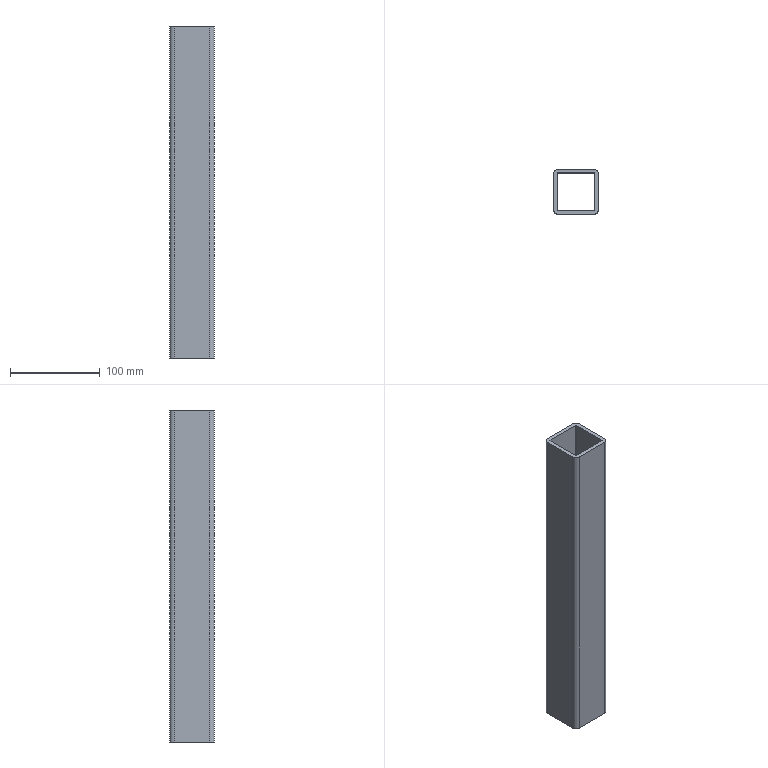Part | STEP file | Square steel 50×50×370 | 1 solid | 18 faces | box 50 x 50 x 370 mm | volume 264697 mm3 | plane 10 | cylinder 8 | commonest cylinder face diameters 2 x4 10 x4
STEP:
#1=CARTESIAN_POINT('',(0.,0.,0.));
#2=DIRECTION('',(0.,0.,1.));
#3=DIRECTION('',(1.,0.,0.));
#4=AXIS2_PLACEMENT_3D('',#1,#2,#3);
#5=CARTESIAN_POINT('',(-25.,-20.,185.));
#6=VERTEX_POINT('',#5);
#7=CARTESIAN_POINT('',(-20.,-25.,185.));
#8=VERTEX_POINT('',#7);
#9=CARTESIAN_POINT('',(-20.,-20.,185.));
#10=DIRECTION('',(0.,0.,1.));
#11=DIRECTION('',(1.,0.,0.));
#12=AXIS2_PLACEMENT_3D('',#9,#10,#11);
#13=CIRCLE('',#12,5.);
#14=CARTESIAN_POINT('',(-20.,-20.,185.));
#15=DIRECTION('',(0.,0.,1.));
#16=DIRECTION('',(1.,0.,0.));
#17=AXIS2_PLACEMENT_3D('',#14,#15,#16);
#18=PLANE('',#17);
#19=CARTESIAN_POINT('',(0.,0.));
#20=DIRECTION('',(1.,0.));
#21=AXIS2_PLACEMENT_2D('',#19,#20);
#22=CIRCLE('',#21,5.);
#23=(GEOMETRIC_REPRESENTATION_CONTEXT(2)PARAMETRIC_REPRESENTATION_CONTEXT()REPRESENTATION_CONTEXT('',''));
#24=DEFINITIONAL_REPRESENTATION('',(#22),#23);
#25=PCURVE('',#18,#24);
#26=CARTESIAN_POINT('',(-20.,-20.,185.));
#27=DIRECTION('',(0.,0.,-1.));
#28=DIRECTION('',(-1.,0.,0.));
#29=AXIS2_PLACEMENT_3D('',#26,#27,#28);
#30=CYLINDRICAL_SURFACE('',#29,5.);
#31=CARTESIAN_POINT('',(9.425,0.));
#32=DIRECTION('',(-1.,0.));
#33=VECTOR('',#32,1.);
#34=LINE('',#31,#33);
#35=(GEOMETRIC_REPRESENTATION_CONTEXT(2)PARAMETRIC_REPRESENTATION_CONTEXT()REPRESENTATION_CONTEXT('',''));
#36=DEFINITIONAL_REPRESENTATION('',(#34),#35);
#37=PCURVE('',#30,#36);
#38=SURFACE_CURVE('',#13,(#25,#37),.PCURVE_S1.);
#39=EDGE_CURVE('',#6,#8,#38,.T.);
#40=ORIENTED_EDGE('',*,*,#39,.T.);
#41=CARTESIAN_POINT('',(20.,-25.,185.));
#42=VERTEX_POINT('',#41);
#43=CARTESIAN_POINT('',(-20.,-25.,185.));
#44=DIRECTION('',(1.,0.,0.));
#45=VECTOR('',#44,1.);
#46=LINE('',#43,#45);
#47=CARTESIAN_POINT('',(0.,-5.));
#48=DIRECTION('',(1.,0.));
#49=VECTOR('',#48,1.);
#50=LINE('',#47,#49);
#51=(GEOMETRIC_REPRESENTATION_CONTEXT(2)PARAMETRIC_REPRESENTATION_CONTEXT()REPRESENTATION_CONTEXT('',''));
#52=DEFINITIONAL_REPRESENTATION('',(#50),#51);
#53=PCURVE('',#18,#52);
#54=CARTESIAN_POINT('',(-20.,-25.,185.));
#55=DIRECTION('',(0.,1.,0.));
#56=DIRECTION('',(0.,0.,1.));
#57=AXIS2_PLACEMENT_3D('',#54,#55,#56);
#58=PLANE('',#57);
#59=CARTESIAN_POINT('',(0.,0.));
#60=DIRECTION('',(0.,1.));
#61=VECTOR('',#60,1.);
#62=LINE('',#59,#61);
#63=(GEOMETRIC_REPRESENTATION_CONTEXT(2)PARAMETRIC_REPRESENTATION_CONTEXT()REPRESENTATION_CONTEXT('',''));
#64=DEFINITIONAL_REPRESENTATION('',(#62),#63);
#65=PCURVE('',#58,#64);
#66=SURFACE_CURVE('',#46,(#53,#65),.PCURVE_S1.);
#67=EDGE_CURVE('',#8,#42,#66,.T.);
#68=ORIENTED_EDGE('',*,*,#67,.T.);
#69=CARTESIAN_POINT('',(25.,-20.,185.));
#70=VERTEX_POINT('',#69);
#71=CARTESIAN_POINT('',(20.,-20.,185.));
#72=DIRECTION('',(0.,0.,1.));
#73=DIRECTION('',(-1.,0.,0.));
#74=AXIS2_PLACEMENT_3D('',#71,#72,#73);
#75=CIRCLE('',#74,5.);
#76=CARTESIAN_POINT('',(40.,0.));
#77=DIRECTION('',(-1.,0.));
#78=AXIS2_PLACEMENT_2D('',#76,#77);
#79=CIRCLE('',#78,5.);
#80=(GEOMETRIC_REPRESENTATION_CONTEXT(2)PARAMETRIC_REPRESENTATION_CONTEXT()REPRESENTATION_CONTEXT('',''));
#81=DEFINITIONAL_REPRESENTATION('',(#79),#80);
#82=PCURVE('',#18,#81);
#83=CARTESIAN_POINT('',(20.,-20.,185.));
#84=DIRECTION('',(0.,0.,-1.));
#85=DIRECTION('',(-1.,0.,0.));
#86=AXIS2_PLACEMENT_3D('',#83,#84,#85);
#87=CYLINDRICAL_SURFACE('',#86,5.);
#88=CARTESIAN_POINT('',(6.283,0.));
#89=DIRECTION('',(-1.,0.));
#90=VECTOR('',#89,1.);
#91=LINE('',#88,#90);
#92=(GEOMETRIC_REPRESENTATION_CONTEXT(2)PARAMETRIC_REPRESENTATION_CONTEXT()REPRESENTATION_CONTEXT('',''));
#93=DEFINITIONAL_REPRESENTATION('',(#91),#92);
#94=PCURVE('',#87,#93);
#95=SURFACE_CURVE('',#75,(#82,#94),.PCURVE_S1.);
#96=EDGE_CURVE('',#42,#70,#95,.T.);
#97=ORIENTED_EDGE('',*,*,#96,.T.);
#98=CARTESIAN_POINT('',(25.,20.,185.));
#99=VERTEX_POINT('',#98);
#100=CARTESIAN_POINT('',(25.,20.,185.));
#101=DIRECTION('',(0.,1.,0.));
#102=VECTOR('',#101,1.);
#103=LINE('',#100,#102);
#104=CARTESIAN_POINT('',(45.,40.));
#105=DIRECTION('',(0.,1.));
#106=VECTOR('',#105,1.);
#107=LINE('',#104,#106);
#108=(GEOMETRIC_REPRESENTATION_CONTEXT(2)PARAMETRIC_REPRESENTATION_CONTEXT()REPRESENTATION_CONTEXT('',''));
#109=DEFINITIONAL_REPRESENTATION('',(#107),#108);
#110=PCURVE('',#18,#109);
#111=CARTESIAN_POINT('',(25.,20.,185.));
#112=DIRECTION('',(-1.,0.,0.));
#113=DIRECTION('',(0.,-1.,0.));
#114=AXIS2_PLACEMENT_3D('',#111,#112,#113);
#115=PLANE('',#114);
#116=CARTESIAN_POINT('',(0.,0.));
#117=DIRECTION('',(-1.,0.));
#118=VECTOR('',#117,1.);
#119=LINE('',#116,#118);
#120=(GEOMETRIC_REPRESENTATION_CONTEXT(2)PARAMETRIC_REPRESENTATION_CONTEXT()REPRESENTATION_CONTEXT('',''));
#121=DEFINITIONAL_REPRESENTATION('',(#119),#120);
#122=PCURVE('',#115,#121);
#123=SURFACE_CURVE('',#103,(#110,#122),.PCURVE_S1.);
#124=EDGE_CURVE('',#70,#99,#123,.T.);
#125=ORIENTED_EDGE('',*,*,#124,.T.);
#126=CARTESIAN_POINT('',(20.,25.,185.));
#127=VERTEX_POINT('',#126);
#128=CARTESIAN_POINT('',(20.,20.,185.));
#129=DIRECTION('',(0.,0.,1.));
#130=DIRECTION('',(1.,0.,0.));
#131=AXIS2_PLACEMENT_3D('',#128,#129,#130);
#132=CIRCLE('',#131,5.);
#133=CARTESIAN_POINT('',(40.,40.));
#134=DIRECTION('',(1.,0.));
#135=AXIS2_PLACEMENT_2D('',#133,#134);
#136=CIRCLE('',#135,5.);
#137=(GEOMETRIC_REPRESENTATION_CONTEXT(2)PARAMETRIC_REPRESENTATION_CONTEXT()REPRESENTATION_CONTEXT('',''));
#138=DEFINITIONAL_REPRESENTATION('',(#136),#137);
#139=PCURVE('',#18,#138);
#140=CARTESIAN_POINT('',(20.,20.,185.));
#141=DIRECTION('',(0.,0.,-1.));
#142=DIRECTION('',(-1.,0.,0.));
#143=AXIS2_PLACEMENT_3D('',#140,#141,#142);
#144=CYLINDRICAL_SURFACE('',#143,5.);
#145=CARTESIAN_POINT('',(3.142,0.));
#146=DIRECTION('',(-1.,0.));
#147=VECTOR('',#146,1.);
#148=LINE('',#145,#147);
#149=(GEOMETRIC_REPRESENTATION_CONTEXT(2)PARAMETRIC_REPRESENTATION_CONTEXT()REPRESENTATION_CONTEXT('',''));
#150=DEFINITIONAL_REPRESENTATION('',(#148),#149);
#151=PCURVE('',#144,#150);
#152=SURFACE_CURVE('',#132,(#139,#151),.PCURVE_S1.);
#153=EDGE_CURVE('',#99,#127,#152,.T.);
#154=ORIENTED_EDGE('',*,*,#153,.T.);
#155=CARTESIAN_POINT('',(-20.,25.,185.));
#156=VERTEX_POINT('',#155);
#157=CARTESIAN_POINT('',(-20.,25.,185.));
#158=DIRECTION('',(-1.,0.,0.));
#159=VECTOR('',#158,1.);
#160=LINE('',#157,#159);
#161=CARTESIAN_POINT('',(0.,45.));
#162=DIRECTION('',(-1.,0.));
#163=VECTOR('',#162,1.);
#164=LINE('',#161,#163);
#165=(GEOMETRIC_REPRESENTATION_CONTEXT(2)PARAMETRIC_REPRESENTATION_CONTEXT()REPRESENTATION_CONTEXT('',''));
#166=DEFINITIONAL_REPRESENTATION('',(#164),#165);
#167=PCURVE('',#18,#166);
#168=CARTESIAN_POINT('',(-20.,25.,185.));
#169=DIRECTION('',(0.,-1.,0.));
#170=DIRECTION('',(0.,0.,-1.));
#171=AXIS2_PLACEMENT_3D('',#168,#169,#170);
#172=PLANE('',#171);
#173=CARTESIAN_POINT('',(0.,0.));
#174=DIRECTION('',(0.,-1.));
#175=VECTOR('',#174,1.);
#176=LINE('',#173,#175);
#177=(GEOMETRIC_REPRESENTATION_CONTEXT(2)PARAMETRIC_REPRESENTATION_CONTEXT()REPRESENTATION_CONTEXT('',''));
#178=DEFINITIONAL_REPRESENTATION('',(#176),#177);
#179=PCURVE('',#172,#178);
#180=SURFACE_CURVE('',#160,(#167,#179),.PCURVE_S1.);
#181=EDGE_CURVE('',#127,#156,#180,.T.);
#182=ORIENTED_EDGE('',*,*,#181,.T.);
#183=CARTESIAN_POINT('',(-25.,20.,185.));
#184=VERTEX_POINT('',#183);
#185=CARTESIAN_POINT('',(-20.,20.,185.));
#186=DIRECTION('',(0.,0.,1.));
#187=DIRECTION('',(-1.,0.,0.));
#188=AXIS2_PLACEMENT_3D('',#185,#186,#187);
#189=CIRCLE('',#188,5.);
#190=CARTESIAN_POINT('',(0.,40.));
#191=DIRECTION('',(-1.,0.));
#192=AXIS2_PLACEMENT_2D('',#190,#191);
#193=CIRCLE('',#192,5.);
#194=(GEOMETRIC_REPRESENTATION_CONTEXT(2)PARAMETRIC_REPRESENTATION_CONTEXT()REPRESENTATION_CONTEXT('',''));
#195=DEFINITIONAL_REPRESENTATION('',(#193),#194);
#196=PCURVE('',#18,#195);
#197=CARTESIAN_POINT('',(-20.,20.,185.));
#198=DIRECTION('',(0.,0.,-1.));
#199=DIRECTION('',(-1.,0.,0.));
#200=AXIS2_PLACEMENT_3D('',#197,#198,#199);
#201=CYLINDRICAL_SURFACE('',#200,5.);
#202=CARTESIAN_POINT('',(6.283,0.));
#203=DIRECTION('',(-1.,0.));
#204=VECTOR('',#203,1.);
#205=LINE('',#202,#204);
#206=(GEOMETRIC_REPRESENTATION_CONTEXT(2)PARAMETRIC_REPRESENTATION_CONTEXT()REPRESENTATION_CONTEXT('',''));
#207=DEFINITIONAL_REPRESENTATION('',(#205),#206);
#208=PCURVE('',#201,#207);
#209=SURFACE_CURVE('',#189,(#196,#208),.PCURVE_S1.);
#210=EDGE_CURVE('',#156,#184,#209,.T.);
#211=ORIENTED_EDGE('',*,*,#210,.T.);
#212=CARTESIAN_POINT('',(-25.,20.,185.));
#213=DIRECTION('',(0.,-1.,0.));
#214=VECTOR('',#213,1.);
#215=LINE('',#212,#214);
#216=CARTESIAN_POINT('',(-5.,40.));
#217=DIRECTION('',(0.,-1.));
#218=VECTOR('',#217,1.);
#219=LINE('',#216,#218);
#220=(GEOMETRIC_REPRESENTATION_CONTEXT(2)PARAMETRIC_REPRESENTATION_CONTEXT()REPRESENTATION_CONTEXT('',''));
#221=DEFINITIONAL_REPRESENTATION('',(#219),#220);
#222=PCURVE('',#18,#221);
#223=CARTESIAN_POINT('',(-25.,20.,185.));
#224=DIRECTION('',(1.,0.,0.));
#225=DIRECTION('',(0.,1.,0.));
#226=AXIS2_PLACEMENT_3D('',#223,#224,#225);
#227=PLANE('',#226);
#228=CARTESIAN_POINT('',(0.,0.));
#229=DIRECTION('',(-1.,0.));
#230=VECTOR('',#229,1.);
#231=LINE('',#228,#230);
#232=(GEOMETRIC_REPRESENTATION_CONTEXT(2)PARAMETRIC_REPRESENTATION_CONTEXT()REPRESENTATION_CONTEXT('',''));
#233=DEFINITIONAL_REPRESENTATION('',(#231),#232);
#234=PCURVE('',#227,#233);
#235=SURFACE_CURVE('',#215,(#222,#234),.PCURVE_S1.);
#236=EDGE_CURVE('',#184,#6,#235,.T.);
#237=ORIENTED_EDGE('',*,*,#236,.T.);
#238=EDGE_LOOP('',(#40,#68,#97,#125,#154,#182,#211,#237));
#239=FACE_BOUND('',#238,.T.);
#240=CARTESIAN_POINT('',(-21.,20.,185.));
#241=VERTEX_POINT('',#240);
#242=CARTESIAN_POINT('',(-21.,-20.,185.));
#243=VERTEX_POINT('',#242);
#244=CARTESIAN_POINT('',(-21.,20.,185.));
#245=DIRECTION('',(0.,-1.,0.));
#246=VECTOR('',#245,1.);
#247=LINE('',#244,#246);
#248=CARTESIAN_POINT('',(-1.,40.));
#249=DIRECTION('',(0.,-1.));
#250=VECTOR('',#249,1.);
#251=LINE('',#248,#250);
#252=(GEOMETRIC_REPRESENTATION_CONTEXT(2)PARAMETRIC_REPRESENTATION_CONTEXT()REPRESENTATION_CONTEXT('',''));
#253=DEFINITIONAL_REPRESENTATION('',(#251),#252);
#254=PCURVE('',#18,#253);
#255=CARTESIAN_POINT('',(-21.,20.,185.));
#256=DIRECTION('',(1.,0.,0.));
#257=DIRECTION('',(0.,1.,0.));
#258=AXIS2_PLACEMENT_3D('',#255,#256,#257);
#259=PLANE('',#258);
#260=CARTESIAN_POINT('',(0.,0.));
#261=DIRECTION('',(-1.,0.));
#262=VECTOR('',#261,1.);
#263=LINE('',#260,#262);
#264=(GEOMETRIC_REPRESENTATION_CONTEXT(2)PARAMETRIC_REPRESENTATION_CONTEXT()REPRESENTATION_CONTEXT('',''));
#265=DEFINITIONAL_REPRESENTATION('',(#263),#264);
#266=PCURVE('',#259,#265);
#267=SURFACE_CURVE('',#247,(#254,#266),.PCURVE_S1.);
#268=EDGE_CURVE('',#241,#243,#267,.T.);
#269=ORIENTED_EDGE('',*,*,#268,.F.);
#270=CARTESIAN_POINT('',(-20.,21.,185.));
#271=VERTEX_POINT('',#270);
#272=CARTESIAN_POINT('',(-20.,20.,185.));
#273=DIRECTION('',(0.,0.,1.));
#274=DIRECTION('',(-1.,0.,0.));
#275=AXIS2_PLACEMENT_3D('',#272,#273,#274);
#276=CIRCLE('',#275,1.);
#277=CARTESIAN_POINT('',(0.,40.));
#278=DIRECTION('',(-1.,0.));
#279=AXIS2_PLACEMENT_2D('',#277,#278);
#280=CIRCLE('',#279,1.);
#281=(GEOMETRIC_REPRESENTATION_CONTEXT(2)PARAMETRIC_REPRESENTATION_CONTEXT()REPRESENTATION_CONTEXT('',''));
#282=DEFINITIONAL_REPRESENTATION('',(#280),#281);
#283=PCURVE('',#18,#282);
#284=CARTESIAN_POINT('',(-20.,20.,185.));
#285=DIRECTION('',(0.,0.,-1.));
#286=DIRECTION('',(-1.,0.,0.));
#287=AXIS2_PLACEMENT_3D('',#284,#285,#286);
#288=CYLINDRICAL_SURFACE('',#287,1.);
#289=CARTESIAN_POINT('',(6.283,0.));
#290=DIRECTION('',(-1.,0.));
#291=VECTOR('',#290,1.);
#292=LINE('',#289,#291);
#293=(GEOMETRIC_REPRESENTATION_CONTEXT(2)PARAMETRIC_REPRESENTATION_CONTEXT()REPRESENTATION_CONTEXT('',''));
#294=DEFINITIONAL_REPRESENTATION('',(#292),#293);
#295=PCURVE('',#288,#294);
#296=SURFACE_CURVE('',#276,(#283,#295),.PCURVE_S1.);
#297=EDGE_CURVE('',#271,#241,#296,.T.);
#298=ORIENTED_EDGE('',*,*,#297,.F.);
#299=CARTESIAN_POINT('',(20.,21.,185.));
#300=VERTEX_POINT('',#299);
#301=CARTESIAN_POINT('',(-20.,21.,185.));
#302=DIRECTION('',(-1.,0.,0.));
#303=VECTOR('',#302,1.);
#304=LINE('',#301,#303);
#305=CARTESIAN_POINT('',(0.,41.));
#306=DIRECTION('',(-1.,0.));
#307=VECTOR('',#306,1.);
#308=LINE('',#305,#307);
#309=(GEOMETRIC_REPRESENTATION_CONTEXT(2)PARAMETRIC_REPRESENTATION_CONTEXT()REPRESENTATION_CONTEXT('',''));
#310=DEFINITIONAL_REPRESENTATION('',(#308),#309);
#311=PCURVE('',#18,#310);
#312=CARTESIAN_POINT('',(-20.,21.,185.));
#313=DIRECTION('',(0.,-1.,0.));
#314=DIRECTION('',(0.,0.,-1.));
#315=AXIS2_PLACEMENT_3D('',#312,#313,#314);
#316=PLANE('',#315);
#317=CARTESIAN_POINT('',(0.,0.));
#318=DIRECTION('',(0.,-1.));
#319=VECTOR('',#318,1.);
#320=LINE('',#317,#319);
#321=(GEOMETRIC_REPRESENTATION_CONTEXT(2)PARAMETRIC_REPRESENTATION_CONTEXT()REPRESENTATION_CONTEXT('',''));
#322=DEFINITIONAL_REPRESENTATION('',(#320),#321);
#323=PCURVE('',#316,#322);
#324=SURFACE_CURVE('',#304,(#311,#323),.PCURVE_S1.);
#325=EDGE_CURVE('',#300,#271,#324,.T.);
#326=ORIENTED_EDGE('',*,*,#325,.F.);
#327=CARTESIAN_POINT('',(21.,20.,185.));
#328=VERTEX_POINT('',#327);
#329=CARTESIAN_POINT('',(20.,20.,185.));
#330=DIRECTION('',(0.,0.,1.));
#331=DIRECTION('',(1.,0.,0.));
#332=AXIS2_PLACEMENT_3D('',#329,#330,#331);
#333=CIRCLE('',#332,1.);
#334=CARTESIAN_POINT('',(40.,40.));
#335=DIRECTION('',(1.,0.));
#336=AXIS2_PLACEMENT_2D('',#334,#335);
#337=CIRCLE('',#336,1.);
#338=(GEOMETRIC_REPRESENTATION_CONTEXT(2)PARAMETRIC_REPRESENTATION_CONTEXT()REPRESENTATION_CONTEXT('',''));
#339=DEFINITIONAL_REPRESENTATION('',(#337),#338);
#340=PCURVE('',#18,#339);
#341=CARTESIAN_POINT('',(20.,20.,185.));
#342=DIRECTION('',(0.,0.,-1.));
#343=DIRECTION('',(-1.,0.,0.));
#344=AXIS2_PLACEMENT_3D('',#341,#342,#343);
#345=CYLINDRICAL_SURFACE('',#344,1.);
#346=CARTESIAN_POINT('',(3.142,0.));
#347=DIRECTION('',(-1.,0.));
#348=VECTOR('',#347,1.);
#349=LINE('',#346,#348);
#350=(GEOMETRIC_REPRESENTATION_CONTEXT(2)PARAMETRIC_REPRESENTATION_CONTEXT()REPRESENTATION_CONTEXT('',''));
#351=DEFINITIONAL_REPRESENTATION('',(#349),#350);
#352=PCURVE('',#345,#351);
#353=SURFACE_CURVE('',#333,(#340,#352),.PCURVE_S1.);
#354=EDGE_CURVE('',#328,#300,#353,.T.);
#355=ORIENTED_EDGE('',*,*,#354,.F.);
#356=CARTESIAN_POINT('',(21.,-20.,185.));
#357=VERTEX_POINT('',#356);
#358=CARTESIAN_POINT('',(21.,20.,185.));
#359=DIRECTION('',(0.,1.,0.));
#360=VECTOR('',#359,1.);
#361=LINE('',#358,#360);
#362=CARTESIAN_POINT('',(41.,40.));
#363=DIRECTION('',(0.,1.));
#364=VECTOR('',#363,1.);
#365=LINE('',#362,#364);
#366=(GEOMETRIC_REPRESENTATION_CONTEXT(2)PARAMETRIC_REPRESENTATION_CONTEXT()REPRESENTATION_CONTEXT('',''));
#367=DEFINITIONAL_REPRESENTATION('',(#365),#366);
#368=PCURVE('',#18,#367);
#369=CARTESIAN_POINT('',(21.,20.,185.));
#370=DIRECTION('',(-1.,0.,0.));
#371=DIRECTION('',(0.,0.,1.));
#372=AXIS2_PLACEMENT_3D('',#369,#370,#371);
#373=PLANE('',#372);
#374=CARTESIAN_POINT('',(0.,0.));
#375=DIRECTION('',(0.,1.));
#376=VECTOR('',#375,1.);
#377=LINE('',#374,#376);
#378=(GEOMETRIC_REPRESENTATION_CONTEXT(2)PARAMETRIC_REPRESENTATION_CONTEXT()REPRESENTATION_CONTEXT('',''));
#379=DEFINITIONAL_REPRESENTATION('',(#377),#378);
#380=PCURVE('',#373,#379);
#381=SURFACE_CURVE('',#361,(#368,#380),.PCURVE_S1.);
#382=EDGE_CURVE('',#357,#328,#381,.T.);
#383=ORIENTED_EDGE('',*,*,#382,.F.);
#384=CARTESIAN_POINT('',(20.,-21.,185.));
#385=VERTEX_POINT('',#384);
#386=CARTESIAN_POINT('',(20.,-20.,185.));
#387=DIRECTION('',(0.,0.,1.));
#388=DIRECTION('',(-1.,0.,0.));
#389=AXIS2_PLACEMENT_3D('',#386,#387,#388);
#390=CIRCLE('',#389,1.);
#391=CARTESIAN_POINT('',(40.,0.));
#392=DIRECTION('',(-1.,0.));
#393=AXIS2_PLACEMENT_2D('',#391,#392);
#394=CIRCLE('',#393,1.);
#395=(GEOMETRIC_REPRESENTATION_CONTEXT(2)PARAMETRIC_REPRESENTATION_CONTEXT()REPRESENTATION_CONTEXT('',''));
#396=DEFINITIONAL_REPRESENTATION('',(#394),#395);
#397=PCURVE('',#18,#396);
#398=CARTESIAN_POINT('',(20.,-20.,185.));
#399=DIRECTION('',(0.,0.,-1.));
#400=DIRECTION('',(-1.,0.,0.));
#401=AXIS2_PLACEMENT_3D('',#398,#399,#400);
#402=CYLINDRICAL_SURFACE('',#401,1.);
#403=CARTESIAN_POINT('',(6.283,0.));
#404=DIRECTION('',(-1.,0.));
#405=VECTOR('',#404,1.);
#406=LINE('',#403,#405);
#407=(GEOMETRIC_REPRESENTATION_CONTEXT(2)PARAMETRIC_REPRESENTATION_CONTEXT()REPRESENTATION_CONTEXT('',''));
#408=DEFINITIONAL_REPRESENTATION('',(#406),#407);
#409=PCURVE('',#402,#408);
#410=SURFACE_CURVE('',#390,(#397,#409),.PCURVE_S1.);
#411=EDGE_CURVE('',#385,#357,#410,.T.);
#412=ORIENTED_EDGE('',*,*,#411,.F.);
#413=CARTESIAN_POINT('',(-20.,-21.,185.));
#414=VERTEX_POINT('',#413);
#415=CARTESIAN_POINT('',(-20.,-21.,185.));
#416=DIRECTION('',(1.,0.,0.));
#417=VECTOR('',#416,1.);
#418=LINE('',#415,#417);
#419=CARTESIAN_POINT('',(0.,-1.));
#420=DIRECTION('',(1.,0.));
#421=VECTOR('',#420,1.);
#422=LINE('',#419,#421);
#423=(GEOMETRIC_REPRESENTATION_CONTEXT(2)PARAMETRIC_REPRESENTATION_CONTEXT()REPRESENTATION_CONTEXT('',''));
#424=DEFINITIONAL_REPRESENTATION('',(#422),#423);
#425=PCURVE('',#18,#424);
#426=CARTESIAN_POINT('',(-20.,-21.,185.));
#427=DIRECTION('',(0.,1.,0.));
#428=DIRECTION('',(0.,0.,1.));
#429=AXIS2_PLACEMENT_3D('',#426,#427,#428);
#430=PLANE('',#429);
#431=CARTESIAN_POINT('',(0.,0.));
#432=DIRECTION('',(0.,1.));
#433=VECTOR('',#432,1.);
#434=LINE('',#431,#433);
#435=(GEOMETRIC_REPRESENTATION_CONTEXT(2)PARAMETRIC_REPRESENTATION_CONTEXT()REPRESENTATION_CONTEXT('',''));
#436=DEFINITIONAL_REPRESENTATION('',(#434),#435);
#437=PCURVE('',#430,#436);
#438=SURFACE_CURVE('',#418,(#425,#437),.PCURVE_S1.);
#439=EDGE_CURVE('',#414,#385,#438,.T.);
#440=ORIENTED_EDGE('',*,*,#439,.F.);
#441=CARTESIAN_POINT('',(-20.,-20.,185.));
#442=DIRECTION('',(0.,0.,1.));
#443=DIRECTION('',(1.,0.,0.));
#444=AXIS2_PLACEMENT_3D('',#441,#442,#443);
#445=CIRCLE('',#444,1.);
#446=CARTESIAN_POINT('',(0.,0.));
#447=DIRECTION('',(1.,0.));
#448=AXIS2_PLACEMENT_2D('',#446,#447);
#449=CIRCLE('',#448,1.);
#450=(GEOMETRIC_REPRESENTATION_CONTEXT(2)PARAMETRIC_REPRESENTATION_CONTEXT()REPRESENTATION_CONTEXT('',''));
#451=DEFINITIONAL_REPRESENTATION('',(#449),#450);
#452=PCURVE('',#18,#451);
#453=CARTESIAN_POINT('',(-20.,-20.,185.));
#454=DIRECTION('',(0.,0.,-1.));
#455=DIRECTION('',(-1.,0.,0.));
#456=AXIS2_PLACEMENT_3D('',#453,#454,#455);
#457=CYLINDRICAL_SURFACE('',#456,1.);
#458=CARTESIAN_POINT('',(9.425,0.));
#459=DIRECTION('',(-1.,0.));
#460=VECTOR('',#459,1.);
#461=LINE('',#458,#460);
#462=(GEOMETRIC_REPRESENTATION_CONTEXT(2)PARAMETRIC_REPRESENTATION_CONTEXT()REPRESENTATION_CONTEXT('',''));
#463=DEFINITIONAL_REPRESENTATION('',(#461),#462);
#464=PCURVE('',#457,#463);
#465=SURFACE_CURVE('',#445,(#452,#464),.PCURVE_S1.);
#466=EDGE_CURVE('',#243,#414,#465,.T.);
#467=ORIENTED_EDGE('',*,*,#466,.F.);
#468=EDGE_LOOP('',(#269,#298,#326,#355,#383,#412,#440,#467));
#469=FACE_BOUND('',#468,.T.);
#470=ADVANCED_FACE('',(#239,#469),#18,.T.);
#471=CARTESIAN_POINT('',(-25.,-20.,-185.));
#472=VERTEX_POINT('',#471);
#473=CARTESIAN_POINT('',(-20.,-25.,-185.));
#474=VERTEX_POINT('',#473);
#475=CARTESIAN_POINT('',(-20.,-20.,-185.));
#476=DIRECTION('',(0.,0.,1.));
#477=DIRECTION('',(1.,0.,0.));
#478=AXIS2_PLACEMENT_3D('',#475,#476,#477);
#479=CIRCLE('',#478,5.);
#480=CARTESIAN_POINT('',(-20.,-20.,-185.));
#481=DIRECTION('',(0.,0.,1.));
#482=DIRECTION('',(1.,0.,0.));
#483=AXIS2_PLACEMENT_3D('',#480,#481,#482);
#484=PLANE('',#483);
#485=CARTESIAN_POINT('',(0.,0.));
#486=DIRECTION('',(1.,0.));
#487=AXIS2_PLACEMENT_2D('',#485,#486);
#488=CIRCLE('',#487,5.);
#489=(GEOMETRIC_REPRESENTATION_CONTEXT(2)PARAMETRIC_REPRESENTATION_CONTEXT()REPRESENTATION_CONTEXT('',''));
#490=DEFINITIONAL_REPRESENTATION('',(#488),#489);
#491=PCURVE('',#484,#490);
#492=CARTESIAN_POINT('',(9.425,370.));
#493=DIRECTION('',(-1.,0.));
#494=VECTOR('',#493,1.);
#495=LINE('',#492,#494);
#496=(GEOMETRIC_REPRESENTATION_CONTEXT(2)PARAMETRIC_REPRESENTATION_CONTEXT()REPRESENTATION_CONTEXT('',''));
#497=DEFINITIONAL_REPRESENTATION('',(#495),#496);
#498=PCURVE('',#30,#497);
#499=SURFACE_CURVE('',#479,(#491,#498),.PCURVE_S1.);
#500=EDGE_CURVE('',#472,#474,#499,.T.);
#501=ORIENTED_EDGE('',*,*,#500,.F.);
#502=CARTESIAN_POINT('',(-25.,20.,-185.));
#503=VERTEX_POINT('',#502);
#504=CARTESIAN_POINT('',(-25.,20.,-185.));
#505=DIRECTION('',(0.,-1.,0.));
#506=VECTOR('',#505,1.);
#507=LINE('',#504,#506);
#508=CARTESIAN_POINT('',(-5.,40.));
#509=DIRECTION('',(0.,-1.));
#510=VECTOR('',#509,1.);
#511=LINE('',#508,#510);
#512=(GEOMETRIC_REPRESENTATION_CONTEXT(2)PARAMETRIC_REPRESENTATION_CONTEXT()REPRESENTATION_CONTEXT('',''));
#513=DEFINITIONAL_REPRESENTATION('',(#511),#512);
#514=PCURVE('',#484,#513);
#515=CARTESIAN_POINT('',(0.,-370.));
#516=DIRECTION('',(-1.,0.));
#517=VECTOR('',#516,1.);
#518=LINE('',#515,#517);
#519=(GEOMETRIC_REPRESENTATION_CONTEXT(2)PARAMETRIC_REPRESENTATION_CONTEXT()REPRESENTATION_CONTEXT('',''));
#520=DEFINITIONAL_REPRESENTATION('',(#518),#519);
#521=PCURVE('',#227,#520);
#522=SURFACE_CURVE('',#507,(#514,#521),.PCURVE_S1.);
#523=EDGE_CURVE('',#503,#472,#522,.T.);
#524=ORIENTED_EDGE('',*,*,#523,.F.);
#525=CARTESIAN_POINT('',(-20.,25.,-185.));
#526=VERTEX_POINT('',#525);
#527=CARTESIAN_POINT('',(-20.,20.,-185.));
#528=DIRECTION('',(0.,0.,1.));
#529=DIRECTION('',(-1.,0.,0.));
#530=AXIS2_PLACEMENT_3D('',#527,#528,#529);
#531=CIRCLE('',#530,5.);
#532=CARTESIAN_POINT('',(0.,40.));
#533=DIRECTION('',(-1.,0.));
#534=AXIS2_PLACEMENT_2D('',#532,#533);
#535=CIRCLE('',#534,5.);
#536=(GEOMETRIC_REPRESENTATION_CONTEXT(2)PARAMETRIC_REPRESENTATION_CONTEXT()REPRESENTATION_CONTEXT('',''));
#537=DEFINITIONAL_REPRESENTATION('',(#535),#536);
#538=PCURVE('',#484,#537);
#539=CARTESIAN_POINT('',(6.283,370.));
#540=DIRECTION('',(-1.,0.));
#541=VECTOR('',#540,1.);
#542=LINE('',#539,#541);
#543=(GEOMETRIC_REPRESENTATION_CONTEXT(2)PARAMETRIC_REPRESENTATION_CONTEXT()REPRESENTATION_CONTEXT('',''));
#544=DEFINITIONAL_REPRESENTATION('',(#542),#543);
#545=PCURVE('',#201,#544);
#546=SURFACE_CURVE('',#531,(#538,#545),.PCURVE_S1.);
#547=EDGE_CURVE('',#526,#503,#546,.T.);
#548=ORIENTED_EDGE('',*,*,#547,.F.);
#549=CARTESIAN_POINT('',(20.,25.,-185.));
#550=VERTEX_POINT('',#549);
#551=CARTESIAN_POINT('',(-20.,25.,-185.));
#552=DIRECTION('',(-1.,0.,0.));
#553=VECTOR('',#552,1.);
#554=LINE('',#551,#553);
#555=CARTESIAN_POINT('',(0.,45.));
#556=DIRECTION('',(-1.,0.));
#557=VECTOR('',#556,1.);
#558=LINE('',#555,#557);
#559=(GEOMETRIC_REPRESENTATION_CONTEXT(2)PARAMETRIC_REPRESENTATION_CONTEXT()REPRESENTATION_CONTEXT('',''));
#560=DEFINITIONAL_REPRESENTATION('',(#558),#559);
#561=PCURVE('',#484,#560);
#562=CARTESIAN_POINT('',(370.,0.));
#563=DIRECTION('',(0.,-1.));
#564=VECTOR('',#563,1.);
#565=LINE('',#562,#564);
#566=(GEOMETRIC_REPRESENTATION_CONTEXT(2)PARAMETRIC_REPRESENTATION_CONTEXT()REPRESENTATION_CONTEXT('',''));
#567=DEFINITIONAL_REPRESENTATION('',(#565),#566);
#568=PCURVE('',#172,#567);
#569=SURFACE_CURVE('',#554,(#561,#568),.PCURVE_S1.);
#570=EDGE_CURVE('',#550,#526,#569,.T.);
#571=ORIENTED_EDGE('',*,*,#570,.F.);
#572=CARTESIAN_POINT('',(25.,20.,-185.));
#573=VERTEX_POINT('',#572);
#574=CARTESIAN_POINT('',(20.,20.,-185.));
#575=DIRECTION('',(0.,0.,1.));
#576=DIRECTION('',(1.,0.,0.));
#577=AXIS2_PLACEMENT_3D('',#574,#575,#576);
#578=CIRCLE('',#577,5.);
#579=CARTESIAN_POINT('',(40.,40.));
#580=DIRECTION('',(1.,0.));
#581=AXIS2_PLACEMENT_2D('',#579,#580);
#582=CIRCLE('',#581,5.);
#583=(GEOMETRIC_REPRESENTATION_CONTEXT(2)PARAMETRIC_REPRESENTATION_CONTEXT()REPRESENTATION_CONTEXT('',''));
#584=DEFINITIONAL_REPRESENTATION('',(#582),#583);
#585=PCURVE('',#484,#584);
#586=CARTESIAN_POINT('',(3.142,370.));
#587=DIRECTION('',(-1.,0.));
#588=VECTOR('',#587,1.);
#589=LINE('',#586,#588);
#590=(GEOMETRIC_REPRESENTATION_CONTEXT(2)PARAMETRIC_REPRESENTATION_CONTEXT()REPRESENTATION_CONTEXT('',''));
#591=DEFINITIONAL_REPRESENTATION('',(#589),#590);
#592=PCURVE('',#144,#591);
#593=SURFACE_CURVE('',#578,(#585,#592),.PCURVE_S1.);
#594=EDGE_CURVE('',#573,#550,#593,.T.);
#595=ORIENTED_EDGE('',*,*,#594,.F.);
#596=CARTESIAN_POINT('',(25.,-20.,-185.));
#597=VERTEX_POINT('',#596);
#598=CARTESIAN_POINT('',(25.,20.,-185.));
#599=DIRECTION('',(0.,1.,0.));
#600=VECTOR('',#599,1.);
#601=LINE('',#598,#600);
#602=CARTESIAN_POINT('',(45.,40.));
#603=DIRECTION('',(0.,1.));
#604=VECTOR('',#603,1.);
#605=LINE('',#602,#604);
#606=(GEOMETRIC_REPRESENTATION_CONTEXT(2)PARAMETRIC_REPRESENTATION_CONTEXT()REPRESENTATION_CONTEXT('',''));
#607=DEFINITIONAL_REPRESENTATION('',(#605),#606);
#608=PCURVE('',#484,#607);
#609=CARTESIAN_POINT('',(0.,-370.));
#610=DIRECTION('',(-1.,0.));
#611=VECTOR('',#610,1.);
#612=LINE('',#609,#611);
#613=(GEOMETRIC_REPRESENTATION_CONTEXT(2)PARAMETRIC_REPRESENTATION_CONTEXT()REPRESENTATION_CONTEXT('',''));
#614=DEFINITIONAL_REPRESENTATION('',(#612),#613);
#615=PCURVE('',#115,#614);
#616=SURFACE_CURVE('',#601,(#608,#615),.PCURVE_S1.);
#617=EDGE_CURVE('',#597,#573,#616,.T.);
#618=ORIENTED_EDGE('',*,*,#617,.F.);
#619=CARTESIAN_POINT('',(20.,-25.,-185.));
#620=VERTEX_POINT('',#619);
#621=CARTESIAN_POINT('',(20.,-20.,-185.));
#622=DIRECTION('',(0.,0.,1.));
#623=DIRECTION('',(-1.,0.,0.));
#624=AXIS2_PLACEMENT_3D('',#621,#622,#623);
#625=CIRCLE('',#624,5.);
#626=CARTESIAN_POINT('',(40.,0.));
#627=DIRECTION('',(-1.,0.));
#628=AXIS2_PLACEMENT_2D('',#626,#627);
#629=CIRCLE('',#628,5.);
#630=(GEOMETRIC_REPRESENTATION_CONTEXT(2)PARAMETRIC_REPRESENTATION_CONTEXT()REPRESENTATION_CONTEXT('',''));
#631=DEFINITIONAL_REPRESENTATION('',(#629),#630);
#632=PCURVE('',#484,#631);
#633=CARTESIAN_POINT('',(6.283,370.));
#634=DIRECTION('',(-1.,0.));
#635=VECTOR('',#634,1.);
#636=LINE('',#633,#635);
#637=(GEOMETRIC_REPRESENTATION_CONTEXT(2)PARAMETRIC_REPRESENTATION_CONTEXT()REPRESENTATION_CONTEXT('',''));
#638=DEFINITIONAL_REPRESENTATION('',(#636),#637);
#639=PCURVE('',#87,#638);
#640=SURFACE_CURVE('',#625,(#632,#639),.PCURVE_S1.);
#641=EDGE_CURVE('',#620,#597,#640,.T.);
#642=ORIENTED_EDGE('',*,*,#641,.F.);
#643=CARTESIAN_POINT('',(-20.,-25.,-185.));
#644=DIRECTION('',(1.,0.,0.));
#645=VECTOR('',#644,1.);
#646=LINE('',#643,#645);
#647=CARTESIAN_POINT('',(0.,-5.));
#648=DIRECTION('',(1.,0.));
#649=VECTOR('',#648,1.);
#650=LINE('',#647,#649);
#651=(GEOMETRIC_REPRESENTATION_CONTEXT(2)PARAMETRIC_REPRESENTATION_CONTEXT()REPRESENTATION_CONTEXT('',''));
#652=DEFINITIONAL_REPRESENTATION('',(#650),#651);
#653=PCURVE('',#484,#652);
#654=CARTESIAN_POINT('',(-370.,0.));
#655=DIRECTION('',(0.,1.));
#656=VECTOR('',#655,1.);
#657=LINE('',#654,#656);
#658=(GEOMETRIC_REPRESENTATION_CONTEXT(2)PARAMETRIC_REPRESENTATION_CONTEXT()REPRESENTATION_CONTEXT('',''));
#659=DEFINITIONAL_REPRESENTATION('',(#657),#658);
#660=PCURVE('',#58,#659);
#661=SURFACE_CURVE('',#646,(#653,#660),.PCURVE_S1.);
#662=EDGE_CURVE('',#474,#620,#661,.T.);
#663=ORIENTED_EDGE('',*,*,#662,.F.);
#664=EDGE_LOOP('',(#501,#524,#548,#571,#595,#618,#642,#663));
#665=FACE_BOUND('',#664,.T.);
#666=CARTESIAN_POINT('',(-20.,21.,-185.));
#667=VERTEX_POINT('',#666);
#668=CARTESIAN_POINT('',(-21.,20.,-185.));
#669=VERTEX_POINT('',#668);
#670=CARTESIAN_POINT('',(-20.,20.,-185.));
#671=DIRECTION('',(0.,0.,1.));
#672=DIRECTION('',(-1.,0.,0.));
#673=AXIS2_PLACEMENT_3D('',#670,#671,#672);
#674=CIRCLE('',#673,1.);
#675=CARTESIAN_POINT('',(0.,40.));
#676=DIRECTION('',(-1.,0.));
#677=AXIS2_PLACEMENT_2D('',#675,#676);
#678=CIRCLE('',#677,1.);
#679=(GEOMETRIC_REPRESENTATION_CONTEXT(2)PARAMETRIC_REPRESENTATION_CONTEXT()REPRESENTATION_CONTEXT('',''));
#680=DEFINITIONAL_REPRESENTATION('',(#678),#679);
#681=PCURVE('',#484,#680);
#682=CARTESIAN_POINT('',(6.283,370.));
#683=DIRECTION('',(-1.,0.));
#684=VECTOR('',#683,1.);
#685=LINE('',#682,#684);
#686=(GEOMETRIC_REPRESENTATION_CONTEXT(2)PARAMETRIC_REPRESENTATION_CONTEXT()REPRESENTATION_CONTEXT('',''));
#687=DEFINITIONAL_REPRESENTATION('',(#685),#686);
#688=PCURVE('',#288,#687);
#689=SURFACE_CURVE('',#674,(#681,#688),.PCURVE_S1.);
#690=EDGE_CURVE('',#667,#669,#689,.T.);
#691=ORIENTED_EDGE('',*,*,#690,.T.);
#692=CARTESIAN_POINT('',(-21.,-20.,-185.));
#693=VERTEX_POINT('',#692);
#694=CARTESIAN_POINT('',(-21.,20.,-185.));
#695=DIRECTION('',(0.,-1.,0.));
#696=VECTOR('',#695,1.);
#697=LINE('',#694,#696);
#698=CARTESIAN_POINT('',(-1.,40.));
#699=DIRECTION('',(0.,-1.));
#700=VECTOR('',#699,1.);
#701=LINE('',#698,#700);
#702=(GEOMETRIC_REPRESENTATION_CONTEXT(2)PARAMETRIC_REPRESENTATION_CONTEXT()REPRESENTATION_CONTEXT('',''));
#703=DEFINITIONAL_REPRESENTATION('',(#701),#702);
#704=PCURVE('',#484,#703);
#705=CARTESIAN_POINT('',(0.,-370.));
#706=DIRECTION('',(-1.,0.));
#707=VECTOR('',#706,1.);
#708=LINE('',#705,#707);
#709=(GEOMETRIC_REPRESENTATION_CONTEXT(2)PARAMETRIC_REPRESENTATION_CONTEXT()REPRESENTATION_CONTEXT('',''));
#710=DEFINITIONAL_REPRESENTATION('',(#708),#709);
#711=PCURVE('',#259,#710);
#712=SURFACE_CURVE('',#697,(#704,#711),.PCURVE_S1.);
#713=EDGE_CURVE('',#669,#693,#712,.T.);
#714=ORIENTED_EDGE('',*,*,#713,.T.);
#715=CARTESIAN_POINT('',(-20.,-21.,-185.));
#716=VERTEX_POINT('',#715);
#717=CARTESIAN_POINT('',(-20.,-20.,-185.));
#718=DIRECTION('',(0.,0.,1.));
#719=DIRECTION('',(1.,0.,0.));
#720=AXIS2_PLACEMENT_3D('',#717,#718,#719);
#721=CIRCLE('',#720,1.);
#722=CARTESIAN_POINT('',(0.,0.));
#723=DIRECTION('',(1.,0.));
#724=AXIS2_PLACEMENT_2D('',#722,#723);
#725=CIRCLE('',#724,1.);
#726=(GEOMETRIC_REPRESENTATION_CONTEXT(2)PARAMETRIC_REPRESENTATION_CONTEXT()REPRESENTATION_CONTEXT('',''));
#727=DEFINITIONAL_REPRESENTATION('',(#725),#726);
#728=PCURVE('',#484,#727);
#729=CARTESIAN_POINT('',(9.425,370.));
#730=DIRECTION('',(-1.,0.));
#731=VECTOR('',#730,1.);
#732=LINE('',#729,#731);
#733=(GEOMETRIC_REPRESENTATION_CONTEXT(2)PARAMETRIC_REPRESENTATION_CONTEXT()REPRESENTATION_CONTEXT('',''));
#734=DEFINITIONAL_REPRESENTATION('',(#732),#733);
#735=PCURVE('',#457,#734);
#736=SURFACE_CURVE('',#721,(#728,#735),.PCURVE_S1.);
#737=EDGE_CURVE('',#693,#716,#736,.T.);
#738=ORIENTED_EDGE('',*,*,#737,.T.);
#739=CARTESIAN_POINT('',(20.,-21.,-185.));
#740=VERTEX_POINT('',#739);
#741=CARTESIAN_POINT('',(-20.,-21.,-185.));
#742=DIRECTION('',(1.,0.,0.));
#743=VECTOR('',#742,1.);
#744=LINE('',#741,#743);
#745=CARTESIAN_POINT('',(0.,-1.));
#746=DIRECTION('',(1.,0.));
#747=VECTOR('',#746,1.);
#748=LINE('',#745,#747);
#749=(GEOMETRIC_REPRESENTATION_CONTEXT(2)PARAMETRIC_REPRESENTATION_CONTEXT()REPRESENTATION_CONTEXT('',''));
#750=DEFINITIONAL_REPRESENTATION('',(#748),#749);
#751=PCURVE('',#484,#750);
#752=CARTESIAN_POINT('',(-370.,0.));
#753=DIRECTION('',(0.,1.));
#754=VECTOR('',#753,1.);
#755=LINE('',#752,#754);
#756=(GEOMETRIC_REPRESENTATION_CONTEXT(2)PARAMETRIC_REPRESENTATION_CONTEXT()REPRESENTATION_CONTEXT('',''));
#757=DEFINITIONAL_REPRESENTATION('',(#755),#756);
#758=PCURVE('',#430,#757);
#759=SURFACE_CURVE('',#744,(#751,#758),.PCURVE_S1.);
#760=EDGE_CURVE('',#716,#740,#759,.T.);
#761=ORIENTED_EDGE('',*,*,#760,.T.);
#762=CARTESIAN_POINT('',(21.,-20.,-185.));
#763=VERTEX_POINT('',#762);
#764=CARTESIAN_POINT('',(20.,-20.,-185.));
#765=DIRECTION('',(0.,0.,1.));
#766=DIRECTION('',(-1.,0.,0.));
#767=AXIS2_PLACEMENT_3D('',#764,#765,#766);
#768=CIRCLE('',#767,1.);
#769=CARTESIAN_POINT('',(40.,0.));
#770=DIRECTION('',(-1.,0.));
#771=AXIS2_PLACEMENT_2D('',#769,#770);
#772=CIRCLE('',#771,1.);
#773=(GEOMETRIC_REPRESENTATION_CONTEXT(2)PARAMETRIC_REPRESENTATION_CONTEXT()REPRESENTATION_CONTEXT('',''));
#774=DEFINITIONAL_REPRESENTATION('',(#772),#773);
#775=PCURVE('',#484,#774);
#776=CARTESIAN_POINT('',(6.283,370.));
#777=DIRECTION('',(-1.,0.));
#778=VECTOR('',#777,1.);
#779=LINE('',#776,#778);
#780=(GEOMETRIC_REPRESENTATION_CONTEXT(2)PARAMETRIC_REPRESENTATION_CONTEXT()REPRESENTATION_CONTEXT('',''));
#781=DEFINITIONAL_REPRESENTATION('',(#779),#780);
#782=PCURVE('',#402,#781);
#783=SURFACE_CURVE('',#768,(#775,#782),.PCURVE_S1.);
#784=EDGE_CURVE('',#740,#763,#783,.T.);
#785=ORIENTED_EDGE('',*,*,#784,.T.);
#786=CARTESIAN_POINT('',(21.,20.,-185.));
#787=VERTEX_POINT('',#786);
#788=CARTESIAN_POINT('',(21.,20.,-185.));
#789=DIRECTION('',(0.,1.,0.));
#790=VECTOR('',#789,1.);
#791=LINE('',#788,#790);
#792=CARTESIAN_POINT('',(41.,40.));
#793=DIRECTION('',(0.,1.));
#794=VECTOR('',#793,1.);
#795=LINE('',#792,#794);
#796=(GEOMETRIC_REPRESENTATION_CONTEXT(2)PARAMETRIC_REPRESENTATION_CONTEXT()REPRESENTATION_CONTEXT('',''));
#797=DEFINITIONAL_REPRESENTATION('',(#795),#796);
#798=PCURVE('',#484,#797);
#799=CARTESIAN_POINT('',(-370.,0.));
#800=DIRECTION('',(0.,1.));
#801=VECTOR('',#800,1.);
#802=LINE('',#799,#801);
#803=(GEOMETRIC_REPRESENTATION_CONTEXT(2)PARAMETRIC_REPRESENTATION_CONTEXT()REPRESENTATION_CONTEXT('',''));
#804=DEFINITIONAL_REPRESENTATION('',(#802),#803);
#805=PCURVE('',#373,#804);
#806=SURFACE_CURVE('',#791,(#798,#805),.PCURVE_S1.);
#807=EDGE_CURVE('',#763,#787,#806,.T.);
#808=ORIENTED_EDGE('',*,*,#807,.T.);
#809=CARTESIAN_POINT('',(20.,21.,-185.));
#810=VERTEX_POINT('',#809);
#811=CARTESIAN_POINT('',(20.,20.,-185.));
#812=DIRECTION('',(0.,0.,1.));
#813=DIRECTION('',(1.,0.,0.));
#814=AXIS2_PLACEMENT_3D('',#811,#812,#813);
#815=CIRCLE('',#814,1.);
#816=CARTESIAN_POINT('',(40.,40.));
#817=DIRECTION('',(1.,0.));
#818=AXIS2_PLACEMENT_2D('',#816,#817);
#819=CIRCLE('',#818,1.);
#820=(GEOMETRIC_REPRESENTATION_CONTEXT(2)PARAMETRIC_REPRESENTATION_CONTEXT()REPRESENTATION_CONTEXT('',''));
#821=DEFINITIONAL_REPRESENTATION('',(#819),#820);
#822=PCURVE('',#484,#821);
#823=CARTESIAN_POINT('',(3.142,370.));
#824=DIRECTION('',(-1.,0.));
#825=VECTOR('',#824,1.);
#826=LINE('',#823,#825);
#827=(GEOMETRIC_REPRESENTATION_CONTEXT(2)PARAMETRIC_REPRESENTATION_CONTEXT()REPRESENTATION_CONTEXT('',''));
#828=DEFINITIONAL_REPRESENTATION('',(#826),#827);
#829=PCURVE('',#345,#828);
#830=SURFACE_CURVE('',#815,(#822,#829),.PCURVE_S1.);
#831=EDGE_CURVE('',#787,#810,#830,.T.);
#832=ORIENTED_EDGE('',*,*,#831,.T.);
#833=CARTESIAN_POINT('',(-20.,21.,-185.));
#834=DIRECTION('',(-1.,0.,0.));
#835=VECTOR('',#834,1.);
#836=LINE('',#833,#835);
#837=CARTESIAN_POINT('',(0.,41.));
#838=DIRECTION('',(-1.,0.));
#839=VECTOR('',#838,1.);
#840=LINE('',#837,#839);
#841=(GEOMETRIC_REPRESENTATION_CONTEXT(2)PARAMETRIC_REPRESENTATION_CONTEXT()REPRESENTATION_CONTEXT('',''));
#842=DEFINITIONAL_REPRESENTATION('',(#840),#841);
#843=PCURVE('',#484,#842);
#844=CARTESIAN_POINT('',(370.,0.));
#845=DIRECTION('',(0.,-1.));
#846=VECTOR('',#845,1.);
#847=LINE('',#844,#846);
#848=(GEOMETRIC_REPRESENTATION_CONTEXT(2)PARAMETRIC_REPRESENTATION_CONTEXT()REPRESENTATION_CONTEXT('',''));
#849=DEFINITIONAL_REPRESENTATION('',(#847),#848);
#850=PCURVE('',#316,#849);
#851=SURFACE_CURVE('',#836,(#843,#850),.PCURVE_S1.);
#852=EDGE_CURVE('',#810,#667,#851,.T.);
#853=ORIENTED_EDGE('',*,*,#852,.T.);
#854=EDGE_LOOP('',(#691,#714,#738,#761,#785,#808,#832,#853));
#855=FACE_BOUND('',#854,.T.);
#856=ADVANCED_FACE('',(#665,#855),#484,.F.);
#857=ORIENTED_EDGE('',*,*,#500,.T.);
#858=CARTESIAN_POINT('',(-20.,-25.,185.));
#859=DIRECTION('',(0.,0.,-1.));
#860=VECTOR('',#859,1.);
#861=LINE('',#858,#860);
#862=CARTESIAN_POINT('',(4.712,0.));
#863=DIRECTION('',(0.,1.));
#864=VECTOR('',#863,1.);
#865=LINE('',#862,#864);
#866=(GEOMETRIC_REPRESENTATION_CONTEXT(2)PARAMETRIC_REPRESENTATION_CONTEXT()REPRESENTATION_CONTEXT('',''));
#867=DEFINITIONAL_REPRESENTATION('',(#865),#866);
#868=PCURVE('',#30,#867);
#869=CARTESIAN_POINT('',(0.,0.));
#870=DIRECTION('',(-1.,0.));
#871=VECTOR('',#870,1.);
#872=LINE('',#869,#871);
#873=(GEOMETRIC_REPRESENTATION_CONTEXT(2)PARAMETRIC_REPRESENTATION_CONTEXT()REPRESENTATION_CONTEXT('',''));
#874=DEFINITIONAL_REPRESENTATION('',(#872),#873);
#875=PCURVE('',#58,#874);
#876=SURFACE_CURVE('',#861,(#868,#875),.PCURVE_S1.);
#877=EDGE_CURVE('',#8,#474,#876,.T.);
#878=ORIENTED_EDGE('',*,*,#877,.F.);
#879=ORIENTED_EDGE('',*,*,#39,.F.);
#880=CARTESIAN_POINT('',(-25.,-20.,185.));
#881=DIRECTION('',(0.,0.,-1.));
#882=VECTOR('',#881,1.);
#883=LINE('',#880,#882);
#884=CARTESIAN_POINT('',(6.283,0.));
#885=DIRECTION('',(0.,1.));
#886=VECTOR('',#885,1.);
#887=LINE('',#884,#886);
#888=(GEOMETRIC_REPRESENTATION_CONTEXT(2)PARAMETRIC_REPRESENTATION_CONTEXT()REPRESENTATION_CONTEXT('',''));
#889=DEFINITIONAL_REPRESENTATION('',(#887),#888);
#890=PCURVE('',#30,#889);
#891=CARTESIAN_POINT('',(-40.,0.));
#892=DIRECTION('',(0.,-1.));
#893=VECTOR('',#892,1.);
#894=LINE('',#891,#893);
#895=(GEOMETRIC_REPRESENTATION_CONTEXT(2)PARAMETRIC_REPRESENTATION_CONTEXT()REPRESENTATION_CONTEXT('',''));
#896=DEFINITIONAL_REPRESENTATION('',(#894),#895);
#897=PCURVE('',#227,#896);
#898=SURFACE_CURVE('',#883,(#890,#897),.PCURVE_S1.);
#899=EDGE_CURVE('',#6,#472,#898,.T.);
#900=ORIENTED_EDGE('',*,*,#899,.T.);
#901=EDGE_LOOP('',(#857,#878,#879,#900));
#902=FACE_BOUND('',#901,.T.);
#903=ADVANCED_FACE('',(#902),#30,.T.);
#904=ORIENTED_EDGE('',*,*,#662,.T.);
#905=CARTESIAN_POINT('',(20.,-25.,185.));
#906=DIRECTION('',(0.,0.,-1.));
#907=VECTOR('',#906,1.);
#908=LINE('',#905,#907);
#909=CARTESIAN_POINT('',(0.,40.));
#910=DIRECTION('',(-1.,0.));
#911=VECTOR('',#910,1.);
#912=LINE('',#909,#911);
#913=(GEOMETRIC_REPRESENTATION_CONTEXT(2)PARAMETRIC_REPRESENTATION_CONTEXT()REPRESENTATION_CONTEXT('',''));
#914=DEFINITIONAL_REPRESENTATION('',(#912),#913);
#915=PCURVE('',#58,#914);
#916=CARTESIAN_POINT('',(4.712,0.));
#917=DIRECTION('',(0.,1.));
#918=VECTOR('',#917,1.);
#919=LINE('',#916,#918);
#920=(GEOMETRIC_REPRESENTATION_CONTEXT(2)PARAMETRIC_REPRESENTATION_CONTEXT()REPRESENTATION_CONTEXT('',''));
#921=DEFINITIONAL_REPRESENTATION('',(#919),#920);
#922=PCURVE('',#87,#921);
#923=SURFACE_CURVE('',#908,(#915,#922),.PCURVE_S1.);
#924=EDGE_CURVE('',#42,#620,#923,.T.);
#925=ORIENTED_EDGE('',*,*,#924,.F.);
#926=ORIENTED_EDGE('',*,*,#67,.F.);
#927=ORIENTED_EDGE('',*,*,#877,.T.);
#928=EDGE_LOOP('',(#904,#925,#926,#927));
#929=FACE_BOUND('',#928,.T.);
#930=ADVANCED_FACE('',(#929),#58,.F.);
#931=ORIENTED_EDGE('',*,*,#641,.T.);
#932=CARTESIAN_POINT('',(25.,-20.,185.));
#933=DIRECTION('',(0.,0.,-1.));
#934=VECTOR('',#933,1.);
#935=LINE('',#932,#934);
#936=CARTESIAN_POINT('',(3.142,0.));
#937=DIRECTION('',(0.,1.));
#938=VECTOR('',#937,1.);
#939=LINE('',#936,#938);
#940=(GEOMETRIC_REPRESENTATION_CONTEXT(2)PARAMETRIC_REPRESENTATION_CONTEXT()REPRESENTATION_CONTEXT('',''));
#941=DEFINITIONAL_REPRESENTATION('',(#939),#940);
#942=PCURVE('',#87,#941);
#943=CARTESIAN_POINT('',(40.,0.));
#944=DIRECTION('',(0.,-1.));
#945=VECTOR('',#944,1.);
#946=LINE('',#943,#945);
#947=(GEOMETRIC_REPRESENTATION_CONTEXT(2)PARAMETRIC_REPRESENTATION_CONTEXT()REPRESENTATION_CONTEXT('',''));
#948=DEFINITIONAL_REPRESENTATION('',(#946),#947);
#949=PCURVE('',#115,#948);
#950=SURFACE_CURVE('',#935,(#942,#949),.PCURVE_S1.);
#951=EDGE_CURVE('',#70,#597,#950,.T.);
#952=ORIENTED_EDGE('',*,*,#951,.F.);
#953=ORIENTED_EDGE('',*,*,#96,.F.);
#954=ORIENTED_EDGE('',*,*,#924,.T.);
#955=EDGE_LOOP('',(#931,#952,#953,#954));
#956=FACE_BOUND('',#955,.T.);
#957=ADVANCED_FACE('',(#956),#87,.T.);
#958=ORIENTED_EDGE('',*,*,#617,.T.);
#959=CARTESIAN_POINT('',(25.,20.,185.));
#960=DIRECTION('',(0.,0.,-1.));
#961=VECTOR('',#960,1.);
#962=LINE('',#959,#961);
#963=CARTESIAN_POINT('',(0.,0.));
#964=DIRECTION('',(0.,-1.));
#965=VECTOR('',#964,1.);
#966=LINE('',#963,#965);
#967=(GEOMETRIC_REPRESENTATION_CONTEXT(2)PARAMETRIC_REPRESENTATION_CONTEXT()REPRESENTATION_CONTEXT('',''));
#968=DEFINITIONAL_REPRESENTATION('',(#966),#967);
#969=PCURVE('',#115,#968);
#970=CARTESIAN_POINT('',(3.142,0.));
#971=DIRECTION('',(0.,1.));
#972=VECTOR('',#971,1.);
#973=LINE('',#970,#972);
#974=(GEOMETRIC_REPRESENTATION_CONTEXT(2)PARAMETRIC_REPRESENTATION_CONTEXT()REPRESENTATION_CONTEXT('',''));
#975=DEFINITIONAL_REPRESENTATION('',(#973),#974);
#976=PCURVE('',#144,#975);
#977=SURFACE_CURVE('',#962,(#969,#976),.PCURVE_S1.);
#978=EDGE_CURVE('',#99,#573,#977,.T.);
#979=ORIENTED_EDGE('',*,*,#978,.F.);
#980=ORIENTED_EDGE('',*,*,#124,.F.);
#981=ORIENTED_EDGE('',*,*,#951,.T.);
#982=EDGE_LOOP('',(#958,#979,#980,#981));
#983=FACE_BOUND('',#982,.T.);
#984=ADVANCED_FACE('',(#983),#115,.F.);
#985=ORIENTED_EDGE('',*,*,#594,.T.);
#986=CARTESIAN_POINT('',(20.,25.,185.));
#987=DIRECTION('',(0.,0.,-1.));
#988=VECTOR('',#987,1.);
#989=LINE('',#986,#988);
#990=CARTESIAN_POINT('',(1.571,0.));
#991=DIRECTION('',(0.,1.));
#992=VECTOR('',#991,1.);
#993=LINE('',#990,#992);
#994=(GEOMETRIC_REPRESENTATION_CONTEXT(2)PARAMETRIC_REPRESENTATION_CONTEXT()REPRESENTATION_CONTEXT('',''));
#995=DEFINITIONAL_REPRESENTATION('',(#993),#994);
#996=PCURVE('',#144,#995);
#997=CARTESIAN_POINT('',(0.,40.));
#998=DIRECTION('',(1.,0.));
#999=VECTOR('',#998,1.);
#1000=LINE('',#997,#999);
#1001=(GEOMETRIC_REPRESENTATION_CONTEXT(2)PARAMETRIC_REPRESENTATION_CONTEXT()REPRESENTATION_CONTEXT('',''));
#1002=DEFINITIONAL_REPRESENTATION('',(#1000),#1001);
#1003=PCURVE('',#172,#1002);
#1004=SURFACE_CURVE('',#989,(#996,#1003),.PCURVE_S1.);
#1005=EDGE_CURVE('',#127,#550,#1004,.T.);
#1006=ORIENTED_EDGE('',*,*,#1005,.F.);
#1007=ORIENTED_EDGE('',*,*,#153,.F.);
#1008=ORIENTED_EDGE('',*,*,#978,.T.);
#1009=EDGE_LOOP('',(#985,#1006,#1007,#1008));
#1010=FACE_BOUND('',#1009,.T.);
#1011=ADVANCED_FACE('',(#1010),#144,.T.);
#1012=ORIENTED_EDGE('',*,*,#570,.T.);
#1013=CARTESIAN_POINT('',(-20.,25.,185.));
#1014=DIRECTION('',(0.,0.,-1.));
#1015=VECTOR('',#1014,1.);
#1016=LINE('',#1013,#1015);
#1017=CARTESIAN_POINT('',(0.,0.));
#1018=DIRECTION('',(1.,0.));
#1019=VECTOR('',#1018,1.);
#1020=LINE('',#1017,#1019);
#1021=(GEOMETRIC_REPRESENTATION_CONTEXT(2)PARAMETRIC_REPRESENTATION_CONTEXT()REPRESENTATION_CONTEXT('',''));
#1022=DEFINITIONAL_REPRESENTATION('',(#1020),#1021);
#1023=PCURVE('',#172,#1022);
#1024=CARTESIAN_POINT('',(1.571,0.));
#1025=DIRECTION('',(0.,1.));
#1026=VECTOR('',#1025,1.);
#1027=LINE('',#1024,#1026);
#1028=(GEOMETRIC_REPRESENTATION_CONTEXT(2)PARAMETRIC_REPRESENTATION_CONTEXT()REPRESENTATION_CONTEXT('',''));
#1029=DEFINITIONAL_REPRESENTATION('',(#1027),#1028);
#1030=PCURVE('',#201,#1029);
#1031=SURFACE_CURVE('',#1016,(#1023,#1030),.PCURVE_S1.);
#1032=EDGE_CURVE('',#156,#526,#1031,.T.);
#1033=ORIENTED_EDGE('',*,*,#1032,.F.);
#1034=ORIENTED_EDGE('',*,*,#181,.F.);
#1035=ORIENTED_EDGE('',*,*,#1005,.T.);
#1036=EDGE_LOOP('',(#1012,#1033,#1034,#1035));
#1037=FACE_BOUND('',#1036,.T.);
#1038=ADVANCED_FACE('',(#1037),#172,.F.);
#1039=ORIENTED_EDGE('',*,*,#547,.T.);
#1040=CARTESIAN_POINT('',(-25.,20.,185.));
#1041=DIRECTION('',(0.,0.,-1.));
#1042=VECTOR('',#1041,1.);
#1043=LINE('',#1040,#1042);
#1044=CARTESIAN_POINT('',(0.,0.));
#1045=DIRECTION('',(0.,1.));
#1046=VECTOR('',#1045,1.);
#1047=LINE('',#1044,#1046);
#1048=(GEOMETRIC_REPRESENTATION_CONTEXT(2)PARAMETRIC_REPRESENTATION_CONTEXT()REPRESENTATION_CONTEXT('',''));
#1049=DEFINITIONAL_REPRESENTATION('',(#1047),#1048);
#1050=PCURVE('',#201,#1049);
#1051=CARTESIAN_POINT('',(0.,0.));
#1052=DIRECTION('',(0.,-1.));
#1053=VECTOR('',#1052,1.);
#1054=LINE('',#1051,#1053);
#1055=(GEOMETRIC_REPRESENTATION_CONTEXT(2)PARAMETRIC_REPRESENTATION_CONTEXT()REPRESENTATION_CONTEXT('',''));
#1056=DEFINITIONAL_REPRESENTATION('',(#1054),#1055);
#1057=PCURVE('',#227,#1056);
#1058=SURFACE_CURVE('',#1043,(#1050,#1057),.PCURVE_S1.);
#1059=EDGE_CURVE('',#184,#503,#1058,.T.);
#1060=ORIENTED_EDGE('',*,*,#1059,.F.);
#1061=ORIENTED_EDGE('',*,*,#210,.F.);
#1062=ORIENTED_EDGE('',*,*,#1032,.T.);
#1063=EDGE_LOOP('',(#1039,#1060,#1061,#1062));
#1064=FACE_BOUND('',#1063,.T.);
#1065=ADVANCED_FACE('',(#1064),#201,.T.);
#1066=ORIENTED_EDGE('',*,*,#523,.T.);
#1067=ORIENTED_EDGE('',*,*,#899,.F.);
#1068=ORIENTED_EDGE('',*,*,#236,.F.);
#1069=ORIENTED_EDGE('',*,*,#1059,.T.);
#1070=EDGE_LOOP('',(#1066,#1067,#1068,#1069));
#1071=FACE_BOUND('',#1070,.T.);
#1072=ADVANCED_FACE('',(#1071),#227,.F.);
#1073=CARTESIAN_POINT('',(-21.,20.,185.));
#1074=DIRECTION('',(0.,0.,-1.));
#1075=VECTOR('',#1074,1.);
#1076=LINE('',#1073,#1075);
#1077=CARTESIAN_POINT('',(0.,0.));
#1078=DIRECTION('',(0.,1.));
#1079=VECTOR('',#1078,1.);
#1080=LINE('',#1077,#1079);
#1081=(GEOMETRIC_REPRESENTATION_CONTEXT(2)PARAMETRIC_REPRESENTATION_CONTEXT()REPRESENTATION_CONTEXT('',''));
#1082=DEFINITIONAL_REPRESENTATION('',(#1080),#1081);
#1083=PCURVE('',#288,#1082);
#1084=CARTESIAN_POINT('',(0.,0.));
#1085=DIRECTION('',(0.,-1.));
#1086=VECTOR('',#1085,1.);
#1087=LINE('',#1084,#1086);
#1088=(GEOMETRIC_REPRESENTATION_CONTEXT(2)PARAMETRIC_REPRESENTATION_CONTEXT()REPRESENTATION_CONTEXT('',''));
#1089=DEFINITIONAL_REPRESENTATION('',(#1087),#1088);
#1090=PCURVE('',#259,#1089);
#1091=SURFACE_CURVE('',#1076,(#1083,#1090),.PCURVE_S1.);
#1092=EDGE_CURVE('',#241,#669,#1091,.T.);
#1093=ORIENTED_EDGE('',*,*,#1092,.F.);
#1094=ORIENTED_EDGE('',*,*,#297,.F.);
#1095=CARTESIAN_POINT('',(-20.,21.,185.));
#1096=DIRECTION('',(0.,0.,-1.));
#1097=VECTOR('',#1096,1.);
#1098=LINE('',#1095,#1097);
#1099=CARTESIAN_POINT('',(1.571,0.));
#1100=DIRECTION('',(0.,1.));
#1101=VECTOR('',#1100,1.);
#1102=LINE('',#1099,#1101);
#1103=(GEOMETRIC_REPRESENTATION_CONTEXT(2)PARAMETRIC_REPRESENTATION_CONTEXT()REPRESENTATION_CONTEXT('',''));
#1104=DEFINITIONAL_REPRESENTATION('',(#1102),#1103);
#1105=PCURVE('',#288,#1104);
#1106=CARTESIAN_POINT('',(0.,0.));
#1107=DIRECTION('',(1.,0.));
#1108=VECTOR('',#1107,1.);
#1109=LINE('',#1106,#1108);
#1110=(GEOMETRIC_REPRESENTATION_CONTEXT(2)PARAMETRIC_REPRESENTATION_CONTEXT()REPRESENTATION_CONTEXT('',''));
#1111=DEFINITIONAL_REPRESENTATION('',(#1109),#1110);
#1112=PCURVE('',#316,#1111);
#1113=SURFACE_CURVE('',#1098,(#1105,#1112),.PCURVE_S1.);
#1114=EDGE_CURVE('',#271,#667,#1113,.T.);
#1115=ORIENTED_EDGE('',*,*,#1114,.T.);
#1116=ORIENTED_EDGE('',*,*,#690,.T.);
#1117=EDGE_LOOP('',(#1093,#1094,#1115,#1116));
#1118=FACE_BOUND('',#1117,.F.);
#1119=ADVANCED_FACE('',(#1118),#288,.F.);
#1120=ORIENTED_EDGE('',*,*,#713,.F.);
#1121=ORIENTED_EDGE('',*,*,#1092,.F.);
#1122=ORIENTED_EDGE('',*,*,#268,.T.);
#1123=CARTESIAN_POINT('',(-21.,-20.,185.));
#1124=DIRECTION('',(0.,0.,-1.));
#1125=VECTOR('',#1124,1.);
#1126=LINE('',#1123,#1125);
#1127=CARTESIAN_POINT('',(-40.,0.));
#1128=DIRECTION('',(0.,-1.));
#1129=VECTOR('',#1128,1.);
#1130=LINE('',#1127,#1129);
#1131=(GEOMETRIC_REPRESENTATION_CONTEXT(2)PARAMETRIC_REPRESENTATION_CONTEXT()REPRESENTATION_CONTEXT('',''));
#1132=DEFINITIONAL_REPRESENTATION('',(#1130),#1131);
#1133=PCURVE('',#259,#1132);
#1134=CARTESIAN_POINT('',(6.283,0.));
#1135=DIRECTION('',(0.,1.));
#1136=VECTOR('',#1135,1.);
#1137=LINE('',#1134,#1136);
#1138=(GEOMETRIC_REPRESENTATION_CONTEXT(2)PARAMETRIC_REPRESENTATION_CONTEXT()REPRESENTATION_CONTEXT('',''));
#1139=DEFINITIONAL_REPRESENTATION('',(#1137),#1138);
#1140=PCURVE('',#457,#1139);
#1141=SURFACE_CURVE('',#1126,(#1133,#1140),.PCURVE_S1.);
#1142=EDGE_CURVE('',#243,#693,#1141,.T.);
#1143=ORIENTED_EDGE('',*,*,#1142,.T.);
#1144=EDGE_LOOP('',(#1120,#1121,#1122,#1143));
#1145=FACE_BOUND('',#1144,.T.);
#1146=ADVANCED_FACE('',(#1145),#259,.T.);
#1147=CARTESIAN_POINT('',(-20.,-21.,185.));
#1148=DIRECTION('',(0.,0.,-1.));
#1149=VECTOR('',#1148,1.);
#1150=LINE('',#1147,#1149);
#1151=CARTESIAN_POINT('',(4.712,0.));
#1152=DIRECTION('',(0.,1.));
#1153=VECTOR('',#1152,1.);
#1154=LINE('',#1151,#1153);
#1155=(GEOMETRIC_REPRESENTATION_CONTEXT(2)PARAMETRIC_REPRESENTATION_CONTEXT()REPRESENTATION_CONTEXT('',''));
#1156=DEFINITIONAL_REPRESENTATION('',(#1154),#1155);
#1157=PCURVE('',#457,#1156);
#1158=CARTESIAN_POINT('',(0.,0.));
#1159=DIRECTION('',(-1.,0.));
#1160=VECTOR('',#1159,1.);
#1161=LINE('',#1158,#1160);
#1162=(GEOMETRIC_REPRESENTATION_CONTEXT(2)PARAMETRIC_REPRESENTATION_CONTEXT()REPRESENTATION_CONTEXT('',''));
#1163=DEFINITIONAL_REPRESENTATION('',(#1161),#1162);
#1164=PCURVE('',#430,#1163);
#1165=SURFACE_CURVE('',#1150,(#1157,#1164),.PCURVE_S1.);
#1166=EDGE_CURVE('',#414,#716,#1165,.T.);
#1167=ORIENTED_EDGE('',*,*,#1166,.F.);
#1168=ORIENTED_EDGE('',*,*,#466,.F.);
#1169=ORIENTED_EDGE('',*,*,#1142,.T.);
#1170=ORIENTED_EDGE('',*,*,#737,.T.);
#1171=EDGE_LOOP('',(#1167,#1168,#1169,#1170));
#1172=FACE_BOUND('',#1171,.F.);
#1173=ADVANCED_FACE('',(#1172),#457,.F.);
#1174=ORIENTED_EDGE('',*,*,#760,.F.);
#1175=ORIENTED_EDGE('',*,*,#1166,.F.);
#1176=ORIENTED_EDGE('',*,*,#439,.T.);
#1177=CARTESIAN_POINT('',(20.,-21.,185.));
#1178=DIRECTION('',(0.,0.,-1.));
#1179=VECTOR('',#1178,1.);
#1180=LINE('',#1177,#1179);
#1181=CARTESIAN_POINT('',(0.,40.));
#1182=DIRECTION('',(-1.,0.));
#1183=VECTOR('',#1182,1.);
#1184=LINE('',#1181,#1183);
#1185=(GEOMETRIC_REPRESENTATION_CONTEXT(2)PARAMETRIC_REPRESENTATION_CONTEXT()REPRESENTATION_CONTEXT('',''));
#1186=DEFINITIONAL_REPRESENTATION('',(#1184),#1185);
#1187=PCURVE('',#430,#1186);
#1188=CARTESIAN_POINT('',(4.712,0.));
#1189=DIRECTION('',(0.,1.));
#1190=VECTOR('',#1189,1.);
#1191=LINE('',#1188,#1190);
#1192=(GEOMETRIC_REPRESENTATION_CONTEXT(2)PARAMETRIC_REPRESENTATION_CONTEXT()REPRESENTATION_CONTEXT('',''));
#1193=DEFINITIONAL_REPRESENTATION('',(#1191),#1192);
#1194=PCURVE('',#402,#1193);
#1195=SURFACE_CURVE('',#1180,(#1187,#1194),.PCURVE_S1.);
#1196=EDGE_CURVE('',#385,#740,#1195,.T.);
#1197=ORIENTED_EDGE('',*,*,#1196,.T.);
#1198=EDGE_LOOP('',(#1174,#1175,#1176,#1197));
#1199=FACE_BOUND('',#1198,.T.);
#1200=ADVANCED_FACE('',(#1199),#430,.T.);
#1201=CARTESIAN_POINT('',(21.,-20.,185.));
#1202=DIRECTION('',(0.,0.,-1.));
#1203=VECTOR('',#1202,1.);
#1204=LINE('',#1201,#1203);
#1205=CARTESIAN_POINT('',(3.142,0.));
#1206=DIRECTION('',(0.,1.));
#1207=VECTOR('',#1206,1.);
#1208=LINE('',#1205,#1207);
#1209=(GEOMETRIC_REPRESENTATION_CONTEXT(2)PARAMETRIC_REPRESENTATION_CONTEXT()REPRESENTATION_CONTEXT('',''));
#1210=DEFINITIONAL_REPRESENTATION('',(#1208),#1209);
#1211=PCURVE('',#402,#1210);
#1212=CARTESIAN_POINT('',(0.,-40.));
#1213=DIRECTION('',(-1.,0.));
#1214=VECTOR('',#1213,1.);
#1215=LINE('',#1212,#1214);
#1216=(GEOMETRIC_REPRESENTATION_CONTEXT(2)PARAMETRIC_REPRESENTATION_CONTEXT()REPRESENTATION_CONTEXT('',''));
#1217=DEFINITIONAL_REPRESENTATION('',(#1215),#1216);
#1218=PCURVE('',#373,#1217);
#1219=SURFACE_CURVE('',#1204,(#1211,#1218),.PCURVE_S1.);
#1220=EDGE_CURVE('',#357,#763,#1219,.T.);
#1221=ORIENTED_EDGE('',*,*,#1220,.F.);
#1222=ORIENTED_EDGE('',*,*,#411,.F.);
#1223=ORIENTED_EDGE('',*,*,#1196,.T.);
#1224=ORIENTED_EDGE('',*,*,#784,.T.);
#1225=EDGE_LOOP('',(#1221,#1222,#1223,#1224));
#1226=FACE_BOUND('',#1225,.F.);
#1227=ADVANCED_FACE('',(#1226),#402,.F.);
#1228=ORIENTED_EDGE('',*,*,#807,.F.);
#1229=ORIENTED_EDGE('',*,*,#1220,.F.);
#1230=ORIENTED_EDGE('',*,*,#382,.T.);
#1231=CARTESIAN_POINT('',(21.,20.,185.));
#1232=DIRECTION('',(0.,0.,-1.));
#1233=VECTOR('',#1232,1.);
#1234=LINE('',#1231,#1233);
#1235=CARTESIAN_POINT('',(0.,0.));
#1236=DIRECTION('',(-1.,0.));
#1237=VECTOR('',#1236,1.);
#1238=LINE('',#1235,#1237);
#1239=(GEOMETRIC_REPRESENTATION_CONTEXT(2)PARAMETRIC_REPRESENTATION_CONTEXT()REPRESENTATION_CONTEXT('',''));
#1240=DEFINITIONAL_REPRESENTATION('',(#1238),#1239);
#1241=PCURVE('',#373,#1240);
#1242=CARTESIAN_POINT('',(3.142,0.));
#1243=DIRECTION('',(0.,1.));
#1244=VECTOR('',#1243,1.);
#1245=LINE('',#1242,#1244);
#1246=(GEOMETRIC_REPRESENTATION_CONTEXT(2)PARAMETRIC_REPRESENTATION_CONTEXT()REPRESENTATION_CONTEXT('',''));
#1247=DEFINITIONAL_REPRESENTATION('',(#1245),#1246);
#1248=PCURVE('',#345,#1247);
#1249=SURFACE_CURVE('',#1234,(#1241,#1248),.PCURVE_S1.);
#1250=EDGE_CURVE('',#328,#787,#1249,.T.);
#1251=ORIENTED_EDGE('',*,*,#1250,.T.);
#1252=EDGE_LOOP('',(#1228,#1229,#1230,#1251));
#1253=FACE_BOUND('',#1252,.T.);
#1254=ADVANCED_FACE('',(#1253),#373,.T.);
#1255=CARTESIAN_POINT('',(20.,21.,185.));
#1256=DIRECTION('',(0.,0.,-1.));
#1257=VECTOR('',#1256,1.);
#1258=LINE('',#1255,#1257);
#1259=CARTESIAN_POINT('',(1.571,0.));
#1260=DIRECTION('',(0.,1.));
#1261=VECTOR('',#1260,1.);
#1262=LINE('',#1259,#1261);
#1263=(GEOMETRIC_REPRESENTATION_CONTEXT(2)PARAMETRIC_REPRESENTATION_CONTEXT()REPRESENTATION_CONTEXT('',''));
#1264=DEFINITIONAL_REPRESENTATION('',(#1262),#1263);
#1265=PCURVE('',#345,#1264);
#1266=CARTESIAN_POINT('',(0.,40.));
#1267=DIRECTION('',(1.,0.));
#1268=VECTOR('',#1267,1.);
#1269=LINE('',#1266,#1268);
#1270=(GEOMETRIC_REPRESENTATION_CONTEXT(2)PARAMETRIC_REPRESENTATION_CONTEXT()REPRESENTATION_CONTEXT('',''));
#1271=DEFINITIONAL_REPRESENTATION('',(#1269),#1270);
#1272=PCURVE('',#316,#1271);
#1273=SURFACE_CURVE('',#1258,(#1265,#1272),.PCURVE_S1.);
#1274=EDGE_CURVE('',#300,#810,#1273,.T.);
#1275=ORIENTED_EDGE('',*,*,#1274,.F.);
#1276=ORIENTED_EDGE('',*,*,#354,.F.);
#1277=ORIENTED_EDGE('',*,*,#1250,.T.);
#1278=ORIENTED_EDGE('',*,*,#831,.T.);
#1279=EDGE_LOOP('',(#1275,#1276,#1277,#1278));
#1280=FACE_BOUND('',#1279,.F.);
#1281=ADVANCED_FACE('',(#1280),#345,.F.);
#1282=ORIENTED_EDGE('',*,*,#852,.F.);
#1283=ORIENTED_EDGE('',*,*,#1274,.F.);
#1284=ORIENTED_EDGE('',*,*,#325,.T.);
#1285=ORIENTED_EDGE('',*,*,#1114,.T.);
#1286=EDGE_LOOP('',(#1282,#1283,#1284,#1285));
#1287=FACE_BOUND('',#1286,.T.);
#1288=ADVANCED_FACE('',(#1287),#316,.T.);
#1289=CLOSED_SHELL('',(#470,#856,#903,#930,#957,#984,#1011,#1038,#1065,#1072,#1119,#1146,#1173,#1200,#1227,#1254,#1281,#1288));
#1290=MANIFOLD_SOLID_BREP('',#1289);
#1291=(LENGTH_UNIT()NAMED_UNIT(*)SI_UNIT(.MILLI.,.METRE.));
#1292=UNCERTAINTY_MEASURE_WITH_UNIT(LENGTH_MEASURE(0.0000001),#1291,'','');
#1293=(NAMED_UNIT(*)PLANE_ANGLE_UNIT()SI_UNIT($,.RADIAN.));
#1294=(NAMED_UNIT(*)SI_UNIT($,.STERADIAN.)SOLID_ANGLE_UNIT());
#1295=(GEOMETRIC_REPRESENTATION_CONTEXT(3)GLOBAL_UNCERTAINTY_ASSIGNED_CONTEXT((#1292))GLOBAL_UNIT_ASSIGNED_CONTEXT((#1291,#1293,#1294))REPRESENTATION_CONTEXT('',''));
#1296=ADVANCED_BREP_SHAPE_REPRESENTATION('',(#4,#1290),#1295);